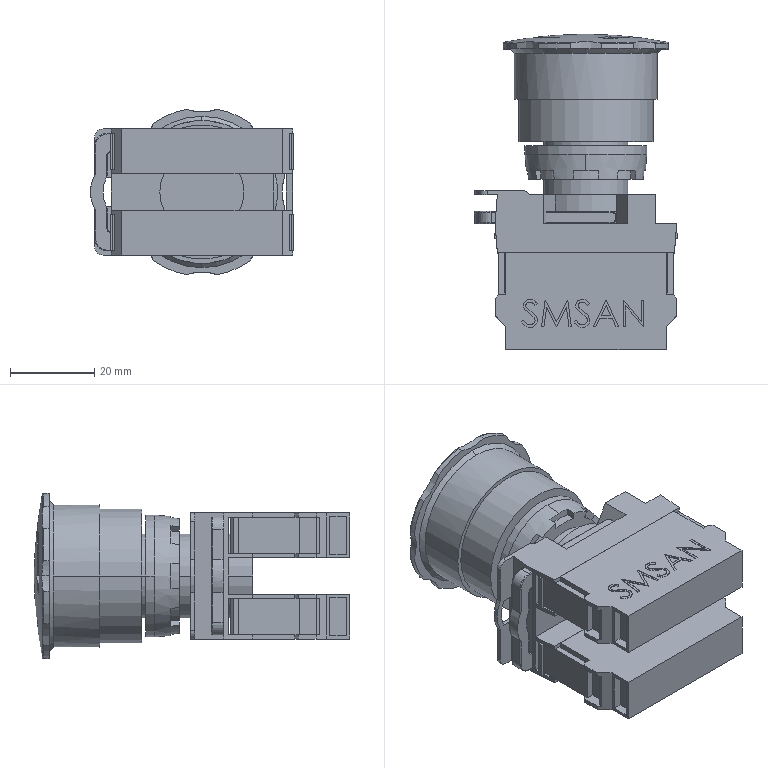Part | STEP file | Emergency stop button[QG115-A1-01ZS╱R] | 5 solids | 458 faces | box 48.3 x 74.961 x 39.345 mm | volume 58947 mm3 | plane 303 | cylinder 90 | spline 59 | cone 6 | commonest cylinder face diameters 0.4 x20 25 x16 20 x15 40 x12 2.5 x4 17 x4